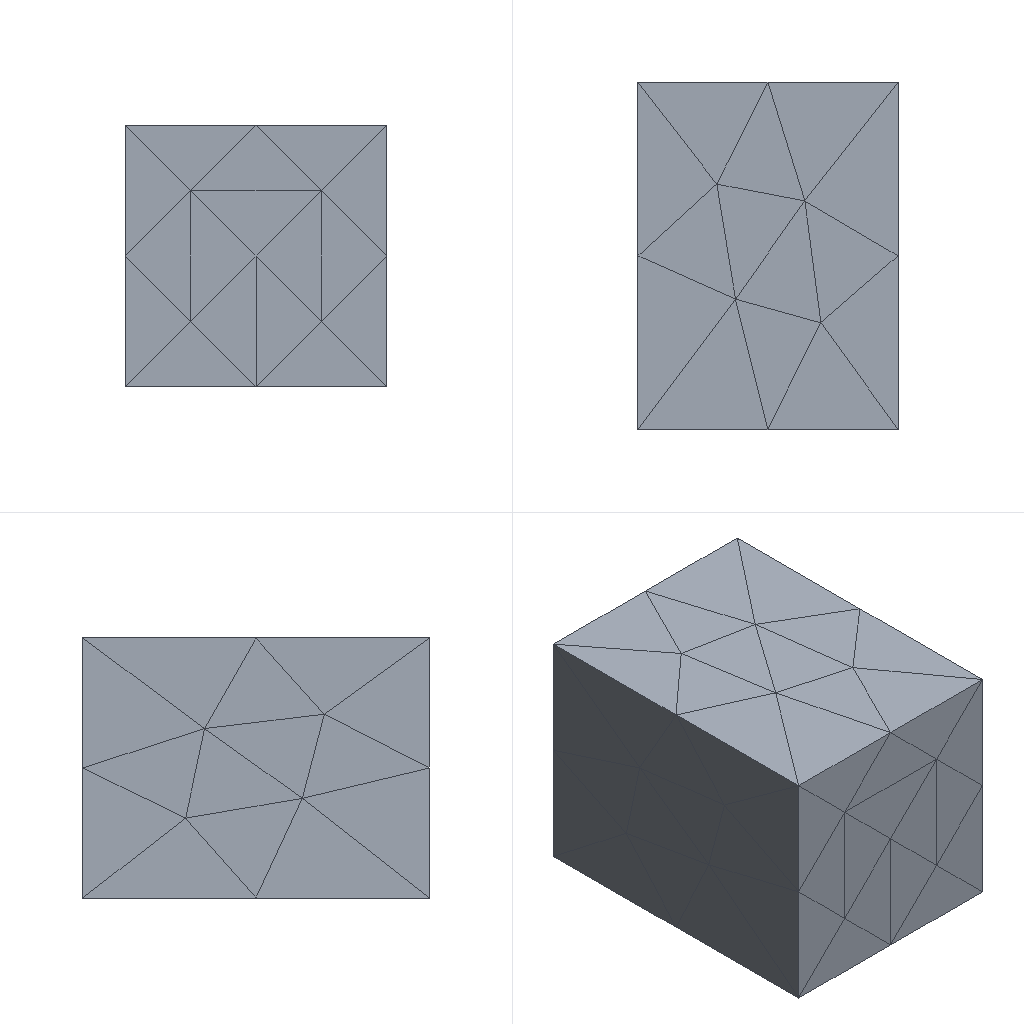Simulation study | ansys mapdl
Set-up summary:
category,name,step,type,value,unit,region
solver,ansys_mapdl
units,mm-N-s-tonne (MPa),,inferred,E=210000 density=
analysis,model,,static
mesh,nodes,,,247
mesh,elements,,,110
element_type,SOLID187,,,110
material,mat 1,,E,210000
material,mat 1,,nu,0.3
load,,model,body load temp,,,all
load,,model,force,"1000 [dir=(0, 0, -1) n=90]",,node list
bc,,model,fixed,"[dofs=UX,UY,UZ n=376]",,node list
Ansys APDL input file, long lists of numbers shortened:
/COM,ANSYS RELEASE 2026 R1           BUILD 26.1      UP20260202       09:08:28
/PREP7
/NOPR
/TITLE,2
ANTYPE, 0
*IF,_CDRDOFF,EQ,1,THEN     !if solid model was read in
_CDRDOFF=             !reset flag, numoffs already performed
*ELSE              !offset database for the following FE model
NUMOFF,NODE,      247
NUMOFF,ELEM,      110
NUMOFF,MAT ,        1
NUMOFF,TYPE,        1
*ENDIF
*SET,_RETURN ,  0.
*SET,_STATUS ,  0.
*SET,_UIQR   ,  90.
*SET,__FLOATPARAMETER__,  247.
DOF,DELETE
ETBLOCK,        1,        1
(2i9,19a9)
        1      187        0        0        0        0        0        0        0        0        0        0        0        0        0        0        0        0        0        0        0
       -1
NBLOCK,6,SOLID,       247,       247
(3i9,6e21.13e3)
        1        0        0 4.1000000000000E+001 8.0000000000000E+000
! (246 more lines like these left out)
N,UNBL,LOC,       -1,
EBLOCK,19,SOLID,       110,       110
(19i10)
         1         1         1         1         0         0         0         0        10         0         1       175       135       178       107       180       181       161       172
! (219 more lines like these left out)
        -1
MPTEMP,UNBL, 1, 1,  0.    ,
MPDATA,UNBL, 1,EX  ,       1, 1,  210000.000    ,
MPTEMP,UNBL, 1, 1,  0.    ,
MPDATA,UNBL, 1,NUXY,       1, 1, 0.3    ,
MPTEMP,UNBL, 1, 1,  0.    ,
MPDATA,UNBL, 1,PRXY,       1, 1, 0.3    ,
EXTOPT,ATTR,      0,      0,      0
EXTOPT,ESIZE,  0,  0.
EXTOPT,ACLEAR,      0
TREF,  0.
IRLF,  0
BFUNIF,TEMP,_TINY
ACEL,  0.    ,  0.    ,  0.
OMEGA,  0.    ,  0.    ,  0.
DOMEGA,  0.    ,  0.    ,  0.
CGLOC,  0.    ,  0.    ,  0.
CGOMEGA,  0.    ,  0.    ,  0.
DCGOMG,  0.    ,  0.    ,  0.
KUSE,     0
TIME,  0.
ALPHAD,  0.
BETAD,  0.
DMPRAT,  0.
DMPSTR,  0.
CRPLIM, 0.1    ,   0
CRPLIM,  0.    ,   1
NCNV,     0, 1.000000000E+12,     0,  0.    ,  0.
NEQIT,     0
ERESX,DEFA
DBLOCK,       376
(i9,a6,2(pg16.9))
        1  UX    0.00000000      0.00000000
! (375 more lines like these left out)
       -1
FBLOCK,        90
(i9,a6,2(pg16.9))
       38  FZ   -11.1111111      0.00000000
! (89 more lines like these left out)
       -1
/GO
FINISH
Results summary:
result,analysis_type_db,,,static,unstated
result,n_sets,,,1,unstated
result,load_steps[0].set,load_step=1,,1,unstated
result,load_steps[0].substep,load_step=1,,1,unstated
result,load_steps[0].time,load_step=1,,1,unstated
result,load_steps[0].freq,load_step=1,,1,unstated
result,load_steps[0].max_usum,load_step=1,,0.0003894,unstated
result,load_steps[0].max_seqv,load_step=1,,9.563,unstated
result,load_steps[0].reaction_sum.FX,load_step=1,,-1.70637e-11,unstated
result,load_steps[0].reaction_sum.FY,load_step=1,,9.11271e-13,unstated
result,load_steps[0].reaction_sum.FZ,load_step=1,,1000,unstated
result,load_steps[0].reaction_sum.MX,load_step=1,,0,unstated
result,load_steps[0].reaction_sum.MY,load_step=1,,0,unstated
result,load_steps[0].reaction_sum.MZ,load_step=1,,0,unstated
result,convergence,,,results present for all listed sets,unstated